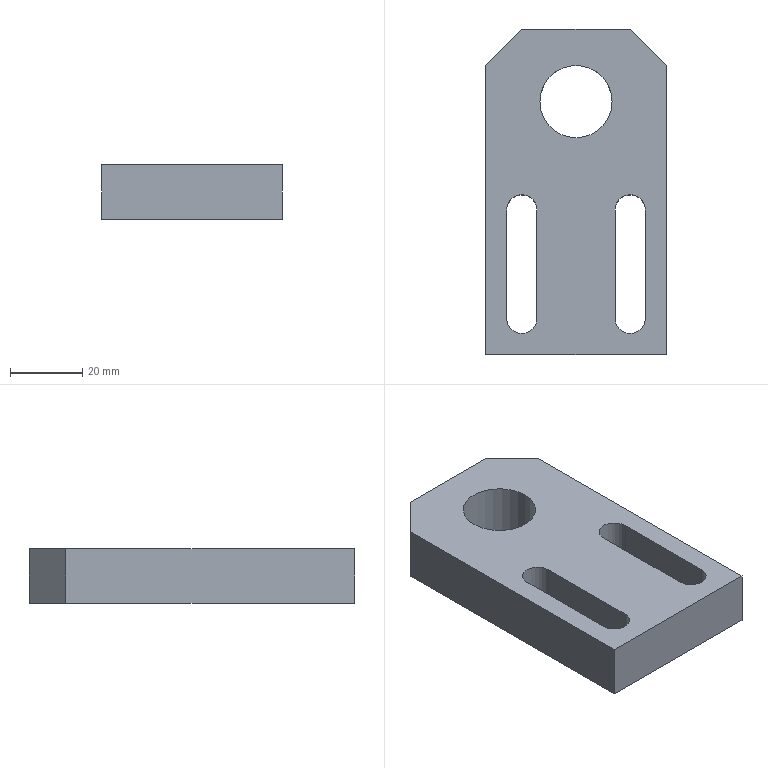Part | SolidWorks | features BaseBody 1 | 1 solid | 18 faces | box 50 x 90 x 15 mm | volume 52065 mm3 | plane 12 | cylinder 6 | commonest cylinder face diameters 8.4 x4 20 x2
STEP:
#1=CARTESIAN_POINT('',(-10.,20.,0.));
#2=VERTEX_POINT('',#1);
#3=CARTESIAN_POINT('',(10.,20.,0.));
#4=VERTEX_POINT('',#3);
#5=CARTESIAN_POINT('',(0.,20.,0.));
#6=DIRECTION('',(0.,0.,1.));
#7=DIRECTION('',(1.,0.,0.));
#8=AXIS2_PLACEMENT_3D('',#5,#6,#7);
#9=CIRCLE('',#8,10.);
#10=EDGE_CURVE('',#2,#4,#9,.T.);
#11=ORIENTED_EDGE('',*,*,#10,.F.);
#12=CARTESIAN_POINT('',(-10.,20.,15.));
#13=VERTEX_POINT('',#12);
#14=CARTESIAN_POINT('',(-10.,20.,0.));
#15=DIRECTION('',(0.,0.,1.));
#16=VECTOR('',#15,1000.);
#17=LINE('',#14,#16);
#18=EDGE_CURVE('',#2,#13,#17,.T.);
#19=ORIENTED_EDGE('',*,*,#18,.T.);
#20=CARTESIAN_POINT('',(10.,20.,15.));
#21=VERTEX_POINT('',#20);
#22=CARTESIAN_POINT('',(0.,20.,15.));
#23=DIRECTION('',(0.,0.,1.));
#24=DIRECTION('',(1.,0.,0.));
#25=AXIS2_PLACEMENT_3D('',#22,#23,#24);
#26=CIRCLE('',#25,10.);
#27=EDGE_CURVE('',#13,#21,#26,.T.);
#28=ORIENTED_EDGE('',*,*,#27,.T.);
#29=CARTESIAN_POINT('',(10.,20.,0.));
#30=DIRECTION('',(0.,0.,1.));
#31=VECTOR('',#30,1000.);
#32=LINE('',#29,#31);
#33=EDGE_CURVE('',#4,#21,#32,.T.);
#34=ORIENTED_EDGE('',*,*,#33,.F.);
#35=EDGE_LOOP('',(#11,#19,#28,#34));
#36=FACE_OUTER_BOUND('',#35,.T.);
#37=CARTESIAN_POINT('',(0.,20.,0.));
#38=DIRECTION('',(0.,0.,1.));
#39=DIRECTION('',(1.,0.,0.));
#40=AXIS2_PLACEMENT_3D('',#37,#38,#39);
#41=CYLINDRICAL_SURFACE('',#40,10.);
#42=ADVANCED_FACE('',(#36),#41,.F.);
#43=CARTESIAN_POINT('',(19.2,-40.,15.));
#44=VERTEX_POINT('',#43);
#45=CARTESIAN_POINT('',(19.2,-10.,15.));
#46=VERTEX_POINT('',#45);
#47=CARTESIAN_POINT('',(19.2,-40.,15.));
#48=DIRECTION('',(0.,1.,0.));
#49=VECTOR('',#48,1000.);
#50=LINE('',#47,#49);
#51=EDGE_CURVE('',#44,#46,#50,.T.);
#52=ORIENTED_EDGE('',*,*,#51,.T.);
#53=CARTESIAN_POINT('',(19.2,-10.,0.));
#54=VERTEX_POINT('',#53);
#55=CARTESIAN_POINT('',(19.2,-10.,0.));
#56=DIRECTION('',(0.,0.,1.));
#57=VECTOR('',#56,1000.);
#58=LINE('',#55,#57);
#59=EDGE_CURVE('',#54,#46,#58,.T.);
#60=ORIENTED_EDGE('',*,*,#59,.F.);
#61=CARTESIAN_POINT('',(19.2,-40.,0.));
#62=VERTEX_POINT('',#61);
#63=CARTESIAN_POINT('',(19.2,-40.,0.));
#64=DIRECTION('',(0.,1.,0.));
#65=VECTOR('',#64,1000.);
#66=LINE('',#63,#65);
#67=EDGE_CURVE('',#62,#54,#66,.T.);
#68=ORIENTED_EDGE('',*,*,#67,.F.);
#69=CARTESIAN_POINT('',(19.2,-40.,0.));
#70=DIRECTION('',(0.,0.,1.));
#71=VECTOR('',#70,1000.);
#72=LINE('',#69,#71);
#73=EDGE_CURVE('',#62,#44,#72,.T.);
#74=ORIENTED_EDGE('',*,*,#73,.T.);
#75=EDGE_LOOP('',(#52,#60,#68,#74));
#76=FACE_OUTER_BOUND('',#75,.T.);
#77=CARTESIAN_POINT('',(19.2,-40.,0.));
#78=DIRECTION('',(1.,0.,0.));
#79=DIRECTION('',(0.,1.,0.));
#80=AXIS2_PLACEMENT_3D('',#77,#78,#79);
#81=PLANE('',#80);
#82=ADVANCED_FACE('',(#76),#81,.F.);
#83=CARTESIAN_POINT('',(10.8,-10.,15.));
#84=VERTEX_POINT('',#83);
#85=CARTESIAN_POINT('',(15.,-10.,15.));
#86=DIRECTION('',(0.,0.,1.));
#87=DIRECTION('',(1.,0.,0.));
#88=AXIS2_PLACEMENT_3D('',#85,#86,#87);
#89=CIRCLE('',#88,4.2);
#90=EDGE_CURVE('',#46,#84,#89,.T.);
#91=ORIENTED_EDGE('',*,*,#90,.T.);
#92=CARTESIAN_POINT('',(10.8,-10.,0.));
#93=VERTEX_POINT('',#92);
#94=CARTESIAN_POINT('',(10.8,-10.,0.));
#95=DIRECTION('',(0.,0.,1.));
#96=VECTOR('',#95,1000.);
#97=LINE('',#94,#96);
#98=EDGE_CURVE('',#93,#84,#97,.T.);
#99=ORIENTED_EDGE('',*,*,#98,.F.);
#100=CARTESIAN_POINT('',(15.,-10.,0.));
#101=DIRECTION('',(0.,0.,1.));
#102=DIRECTION('',(1.,0.,0.));
#103=AXIS2_PLACEMENT_3D('',#100,#101,#102);
#104=CIRCLE('',#103,4.2);
#105=EDGE_CURVE('',#54,#93,#104,.T.);
#106=ORIENTED_EDGE('',*,*,#105,.F.);
#107=ORIENTED_EDGE('',*,*,#59,.T.);
#108=EDGE_LOOP('',(#91,#99,#106,#107));
#109=FACE_OUTER_BOUND('',#108,.T.);
#110=CARTESIAN_POINT('',(15.,-10.,0.));
#111=DIRECTION('',(0.,0.,1.));
#112=DIRECTION('',(1.,0.,0.));
#113=AXIS2_PLACEMENT_3D('',#110,#111,#112);
#114=CYLINDRICAL_SURFACE('',#113,4.2);
#115=ADVANCED_FACE('',(#109),#114,.F.);
#116=CARTESIAN_POINT('',(10.8,-40.,15.));
#117=VERTEX_POINT('',#116);
#118=CARTESIAN_POINT('',(10.8,-40.,15.));
#119=DIRECTION('',(0.,-1.,0.));
#120=VECTOR('',#119,1000.);
#121=LINE('',#118,#120);
#122=EDGE_CURVE('',#84,#117,#121,.T.);
#123=ORIENTED_EDGE('',*,*,#122,.T.);
#124=CARTESIAN_POINT('',(10.8,-40.,0.));
#125=VERTEX_POINT('',#124);
#126=CARTESIAN_POINT('',(10.8,-40.,0.));
#127=DIRECTION('',(0.,0.,1.));
#128=VECTOR('',#127,1000.);
#129=LINE('',#126,#128);
#130=EDGE_CURVE('',#125,#117,#129,.T.);
#131=ORIENTED_EDGE('',*,*,#130,.F.);
#132=CARTESIAN_POINT('',(10.8,-40.,0.));
#133=DIRECTION('',(0.,-1.,0.));
#134=VECTOR('',#133,1000.);
#135=LINE('',#132,#134);
#136=EDGE_CURVE('',#93,#125,#135,.T.);
#137=ORIENTED_EDGE('',*,*,#136,.F.);
#138=ORIENTED_EDGE('',*,*,#98,.T.);
#139=EDGE_LOOP('',(#123,#131,#137,#138));
#140=FACE_OUTER_BOUND('',#139,.T.);
#141=CARTESIAN_POINT('',(10.8,-40.,0.));
#142=DIRECTION('',(-1.,0.,0.));
#143=DIRECTION('',(0.,1.,0.));
#144=AXIS2_PLACEMENT_3D('',#141,#142,#143);
#145=PLANE('',#144);
#146=ADVANCED_FACE('',(#140),#145,.F.);
#147=CARTESIAN_POINT('',(15.,-40.,15.));
#148=DIRECTION('',(0.,0.,1.));
#149=DIRECTION('',(1.,0.,0.));
#150=AXIS2_PLACEMENT_3D('',#147,#148,#149);
#151=CIRCLE('',#150,4.2);
#152=EDGE_CURVE('',#117,#44,#151,.T.);
#153=ORIENTED_EDGE('',*,*,#152,.T.);
#154=ORIENTED_EDGE('',*,*,#73,.F.);
#155=CARTESIAN_POINT('',(15.,-40.,0.));
#156=DIRECTION('',(0.,0.,1.));
#157=DIRECTION('',(1.,0.,0.));
#158=AXIS2_PLACEMENT_3D('',#155,#156,#157);
#159=CIRCLE('',#158,4.2);
#160=EDGE_CURVE('',#125,#62,#159,.T.);
#161=ORIENTED_EDGE('',*,*,#160,.F.);
#162=ORIENTED_EDGE('',*,*,#130,.T.);
#163=EDGE_LOOP('',(#153,#154,#161,#162));
#164=FACE_OUTER_BOUND('',#163,.T.);
#165=CARTESIAN_POINT('',(15.,-40.,0.));
#166=DIRECTION('',(0.,0.,1.));
#167=DIRECTION('',(1.,0.,0.));
#168=AXIS2_PLACEMENT_3D('',#165,#166,#167);
#169=CYLINDRICAL_SURFACE('',#168,4.2);
#170=ADVANCED_FACE('',(#164),#169,.F.);
#171=CARTESIAN_POINT('',(-10.8,-40.,15.));
#172=VERTEX_POINT('',#171);
#173=CARTESIAN_POINT('',(-10.8,-10.,15.));
#174=VERTEX_POINT('',#173);
#175=CARTESIAN_POINT('',(-10.8,-40.,15.));
#176=DIRECTION('',(0.,1.,0.));
#177=VECTOR('',#176,1000.);
#178=LINE('',#175,#177);
#179=EDGE_CURVE('',#172,#174,#178,.T.);
#180=ORIENTED_EDGE('',*,*,#179,.T.);
#181=CARTESIAN_POINT('',(-10.8,-10.,0.));
#182=VERTEX_POINT('',#181);
#183=CARTESIAN_POINT('',(-10.8,-10.,0.));
#184=DIRECTION('',(0.,0.,1.));
#185=VECTOR('',#184,1000.);
#186=LINE('',#183,#185);
#187=EDGE_CURVE('',#182,#174,#186,.T.);
#188=ORIENTED_EDGE('',*,*,#187,.F.);
#189=CARTESIAN_POINT('',(-10.8,-40.,0.));
#190=VERTEX_POINT('',#189);
#191=CARTESIAN_POINT('',(-10.8,-40.,0.));
#192=DIRECTION('',(0.,1.,0.));
#193=VECTOR('',#192,1000.);
#194=LINE('',#191,#193);
#195=EDGE_CURVE('',#190,#182,#194,.T.);
#196=ORIENTED_EDGE('',*,*,#195,.F.);
#197=CARTESIAN_POINT('',(-10.8,-40.,0.));
#198=DIRECTION('',(0.,0.,1.));
#199=VECTOR('',#198,1000.);
#200=LINE('',#197,#199);
#201=EDGE_CURVE('',#190,#172,#200,.T.);
#202=ORIENTED_EDGE('',*,*,#201,.T.);
#203=EDGE_LOOP('',(#180,#188,#196,#202));
#204=FACE_OUTER_BOUND('',#203,.T.);
#205=CARTESIAN_POINT('',(-10.8,-40.,0.));
#206=DIRECTION('',(1.,0.,0.));
#207=DIRECTION('',(0.,1.,0.));
#208=AXIS2_PLACEMENT_3D('',#205,#206,#207);
#209=PLANE('',#208);
#210=ADVANCED_FACE('',(#204),#209,.F.);
#211=CARTESIAN_POINT('',(-19.2,-10.,15.));
#212=VERTEX_POINT('',#211);
#213=CARTESIAN_POINT('',(-15.,-10.,15.));
#214=DIRECTION('',(0.,0.,1.));
#215=DIRECTION('',(1.,0.,0.));
#216=AXIS2_PLACEMENT_3D('',#213,#214,#215);
#217=CIRCLE('',#216,4.2);
#218=EDGE_CURVE('',#174,#212,#217,.T.);
#219=ORIENTED_EDGE('',*,*,#218,.T.);
#220=CARTESIAN_POINT('',(-19.2,-10.,0.));
#221=VERTEX_POINT('',#220);
#222=CARTESIAN_POINT('',(-19.2,-10.,0.));
#223=DIRECTION('',(0.,0.,1.));
#224=VECTOR('',#223,1000.);
#225=LINE('',#222,#224);
#226=EDGE_CURVE('',#221,#212,#225,.T.);
#227=ORIENTED_EDGE('',*,*,#226,.F.);
#228=CARTESIAN_POINT('',(-15.,-10.,0.));
#229=DIRECTION('',(0.,0.,1.));
#230=DIRECTION('',(1.,0.,0.));
#231=AXIS2_PLACEMENT_3D('',#228,#229,#230);
#232=CIRCLE('',#231,4.2);
#233=EDGE_CURVE('',#182,#221,#232,.T.);
#234=ORIENTED_EDGE('',*,*,#233,.F.);
#235=ORIENTED_EDGE('',*,*,#187,.T.);
#236=EDGE_LOOP('',(#219,#227,#234,#235));
#237=FACE_OUTER_BOUND('',#236,.T.);
#238=CARTESIAN_POINT('',(-15.,-10.,0.));
#239=DIRECTION('',(0.,0.,1.));
#240=DIRECTION('',(1.,0.,0.));
#241=AXIS2_PLACEMENT_3D('',#238,#239,#240);
#242=CYLINDRICAL_SURFACE('',#241,4.2);
#243=ADVANCED_FACE('',(#237),#242,.F.);
#244=CARTESIAN_POINT('',(-19.2,-40.,15.));
#245=VERTEX_POINT('',#244);
#246=CARTESIAN_POINT('',(-19.2,-40.,15.));
#247=DIRECTION('',(0.,-1.,0.));
#248=VECTOR('',#247,1000.);
#249=LINE('',#246,#248);
#250=EDGE_CURVE('',#212,#245,#249,.T.);
#251=ORIENTED_EDGE('',*,*,#250,.T.);
#252=CARTESIAN_POINT('',(-19.2,-40.,0.));
#253=VERTEX_POINT('',#252);
#254=CARTESIAN_POINT('',(-19.2,-40.,0.));
#255=DIRECTION('',(0.,0.,1.));
#256=VECTOR('',#255,1000.);
#257=LINE('',#254,#256);
#258=EDGE_CURVE('',#253,#245,#257,.T.);
#259=ORIENTED_EDGE('',*,*,#258,.F.);
#260=CARTESIAN_POINT('',(-19.2,-40.,0.));
#261=DIRECTION('',(0.,-1.,0.));
#262=VECTOR('',#261,1000.);
#263=LINE('',#260,#262);
#264=EDGE_CURVE('',#221,#253,#263,.T.);
#265=ORIENTED_EDGE('',*,*,#264,.F.);
#266=ORIENTED_EDGE('',*,*,#226,.T.);
#267=EDGE_LOOP('',(#251,#259,#265,#266));
#268=FACE_OUTER_BOUND('',#267,.T.);
#269=CARTESIAN_POINT('',(-19.2,-40.,0.));
#270=DIRECTION('',(-1.,0.,0.));
#271=DIRECTION('',(0.,1.,0.));
#272=AXIS2_PLACEMENT_3D('',#269,#270,#271);
#273=PLANE('',#272);
#274=ADVANCED_FACE('',(#268),#273,.F.);
#275=CARTESIAN_POINT('',(-15.,-40.,15.));
#276=DIRECTION('',(0.,0.,1.));
#277=DIRECTION('',(1.,0.,0.));
#278=AXIS2_PLACEMENT_3D('',#275,#276,#277);
#279=CIRCLE('',#278,4.2);
#280=EDGE_CURVE('',#245,#172,#279,.T.);
#281=ORIENTED_EDGE('',*,*,#280,.T.);
#282=ORIENTED_EDGE('',*,*,#201,.F.);
#283=CARTESIAN_POINT('',(-15.,-40.,0.));
#284=DIRECTION('',(0.,0.,1.));
#285=DIRECTION('',(1.,0.,0.));
#286=AXIS2_PLACEMENT_3D('',#283,#284,#285);
#287=CIRCLE('',#286,4.2);
#288=EDGE_CURVE('',#253,#190,#287,.T.);
#289=ORIENTED_EDGE('',*,*,#288,.F.);
#290=ORIENTED_EDGE('',*,*,#258,.T.);
#291=EDGE_LOOP('',(#281,#282,#289,#290));
#292=FACE_OUTER_BOUND('',#291,.T.);
#293=CARTESIAN_POINT('',(-15.,-40.,0.));
#294=DIRECTION('',(0.,0.,1.));
#295=DIRECTION('',(1.,0.,0.));
#296=AXIS2_PLACEMENT_3D('',#293,#294,#295);
#297=CYLINDRICAL_SURFACE('',#296,4.2);
#298=ADVANCED_FACE('',(#292),#297,.F.);
#299=CARTESIAN_POINT('',(-25.,-50.,15.));
#300=VERTEX_POINT('',#299);
#301=CARTESIAN_POINT('',(-25.,-50.,0.));
#302=VERTEX_POINT('',#301);
#303=CARTESIAN_POINT('',(-25.,-50.,15.));
#304=DIRECTION('',(0.,0.,-1.));
#305=VECTOR('',#304,1000.);
#306=LINE('',#303,#305);
#307=EDGE_CURVE('',#300,#302,#306,.T.);
#308=ORIENTED_EDGE('',*,*,#307,.T.);
#309=CARTESIAN_POINT('',(25.,-50.,0.));
#310=VERTEX_POINT('',#309);
#311=CARTESIAN_POINT('',(-25.,-50.,0.));
#312=DIRECTION('',(1.,0.,0.));
#313=VECTOR('',#312,1000.);
#314=LINE('',#311,#313);
#315=EDGE_CURVE('',#302,#310,#314,.T.);
#316=ORIENTED_EDGE('',*,*,#315,.T.);
#317=CARTESIAN_POINT('',(25.,-50.,15.));
#318=VERTEX_POINT('',#317);
#319=CARTESIAN_POINT('',(25.,-50.,0.));
#320=DIRECTION('',(0.,0.,1.));
#321=VECTOR('',#320,1000.);
#322=LINE('',#319,#321);
#323=EDGE_CURVE('',#310,#318,#322,.T.);
#324=ORIENTED_EDGE('',*,*,#323,.T.);
#325=CARTESIAN_POINT('',(25.,-50.,15.));
#326=DIRECTION('',(-1.,0.,0.));
#327=VECTOR('',#326,1000.);
#328=LINE('',#325,#327);
#329=EDGE_CURVE('',#318,#300,#328,.T.);
#330=ORIENTED_EDGE('',*,*,#329,.T.);
#331=EDGE_LOOP('',(#308,#316,#324,#330));
#332=FACE_OUTER_BOUND('',#331,.T.);
#333=CARTESIAN_POINT('',(0.,-50.,0.));
#334=DIRECTION('',(0.,-1.,0.));
#335=DIRECTION('',(0.,0.,-1.));
#336=AXIS2_PLACEMENT_3D('',#333,#334,#335);
#337=PLANE('',#336);
#338=ADVANCED_FACE('',(#332),#337,.T.);
#339=CARTESIAN_POINT('',(-15.,40.,15.));
#340=VERTEX_POINT('',#339);
#341=CARTESIAN_POINT('',(-25.,30.,15.));
#342=VERTEX_POINT('',#341);
#343=CARTESIAN_POINT('',(-27.5,27.5,15.));
#344=DIRECTION('',(-0.7071,-0.7071,0.));
#345=VECTOR('',#344,1000.);
#346=LINE('',#343,#345);
#347=EDGE_CURVE('',#340,#342,#346,.T.);
#348=ORIENTED_EDGE('',*,*,#347,.F.);
#349=CARTESIAN_POINT('',(-15.,40.,0.));
#350=VERTEX_POINT('',#349);
#351=CARTESIAN_POINT('',(-15.,40.,15.));
#352=DIRECTION('',(0.,0.,1.));
#353=VECTOR('',#352,1000.);
#354=LINE('',#351,#353);
#355=EDGE_CURVE('',#350,#340,#354,.T.);
#356=ORIENTED_EDGE('',*,*,#355,.F.);
#357=CARTESIAN_POINT('',(-25.,30.,0.));
#358=VERTEX_POINT('',#357);
#359=CARTESIAN_POINT('',(-25.,30.,0.));
#360=DIRECTION('',(0.7071,0.7071,0.));
#361=VECTOR('',#360,1000.);
#362=LINE('',#359,#361);
#363=EDGE_CURVE('',#358,#350,#362,.T.);
#364=ORIENTED_EDGE('',*,*,#363,.F.);
#365=CARTESIAN_POINT('',(-25.,30.,15.));
#366=DIRECTION('',(0.,0.,-1.));
#367=VECTOR('',#366,1000.);
#368=LINE('',#365,#367);
#369=EDGE_CURVE('',#342,#358,#368,.T.);
#370=ORIENTED_EDGE('',*,*,#369,.F.);
#371=EDGE_LOOP('',(#348,#356,#364,#370));
#372=FACE_OUTER_BOUND('',#371,.T.);
#373=CARTESIAN_POINT('',(-25.,30.,15.));
#374=DIRECTION('',(0.7071,-0.7071,0.));
#375=DIRECTION('',(0.,0.,-1.));
#376=AXIS2_PLACEMENT_3D('',#373,#374,#375);
#377=PLANE('',#376);
#378=ADVANCED_FACE('',(#372),#377,.F.);
#379=CARTESIAN_POINT('',(25.,30.,15.));
#380=VERTEX_POINT('',#379);
#381=CARTESIAN_POINT('',(15.,40.,15.));
#382=VERTEX_POINT('',#381);
#383=CARTESIAN_POINT('',(27.5,27.5,15.));
#384=DIRECTION('',(-0.7071,0.7071,0.));
#385=VECTOR('',#384,1000.);
#386=LINE('',#383,#385);
#387=EDGE_CURVE('',#380,#382,#386,.T.);
#388=ORIENTED_EDGE('',*,*,#387,.F.);
#389=CARTESIAN_POINT('',(25.,30.,0.));
#390=VERTEX_POINT('',#389);
#391=CARTESIAN_POINT('',(25.,30.,15.));
#392=DIRECTION('',(0.,0.,1.));
#393=VECTOR('',#392,1000.);
#394=LINE('',#391,#393);
#395=EDGE_CURVE('',#390,#380,#394,.T.);
#396=ORIENTED_EDGE('',*,*,#395,.F.);
#397=CARTESIAN_POINT('',(15.,40.,0.));
#398=VERTEX_POINT('',#397);
#399=CARTESIAN_POINT('',(15.,40.,0.));
#400=DIRECTION('',(0.7071,-0.7071,0.));
#401=VECTOR('',#400,1000.);
#402=LINE('',#399,#401);
#403=EDGE_CURVE('',#398,#390,#402,.T.);
#404=ORIENTED_EDGE('',*,*,#403,.F.);
#405=CARTESIAN_POINT('',(15.,40.,15.));
#406=DIRECTION('',(0.,0.,-1.));
#407=VECTOR('',#406,1000.);
#408=LINE('',#405,#407);
#409=EDGE_CURVE('',#382,#398,#408,.T.);
#410=ORIENTED_EDGE('',*,*,#409,.F.);
#411=EDGE_LOOP('',(#388,#396,#404,#410));
#412=FACE_OUTER_BOUND('',#411,.T.);
#413=CARTESIAN_POINT('',(15.,40.,15.));
#414=DIRECTION('',(-0.7071,-0.7071,0.));
#415=DIRECTION('',(-0.7071,0.7071,0.));
#416=AXIS2_PLACEMENT_3D('',#413,#414,#415);
#417=PLANE('',#416);
#418=ADVANCED_FACE('',(#412),#417,.F.);
#419=CARTESIAN_POINT('',(0.,20.,0.));
#420=DIRECTION('',(0.,0.,1.));
#421=DIRECTION('',(1.,0.,0.));
#422=AXIS2_PLACEMENT_3D('',#419,#420,#421);
#423=CIRCLE('',#422,10.);
#424=EDGE_CURVE('',#4,#2,#423,.T.);
#425=ORIENTED_EDGE('',*,*,#424,.T.);
#426=ORIENTED_EDGE('',*,*,#10,.T.);
#427=EDGE_LOOP('',(#425,#426));
#428=FACE_BOUND('',#427,.T.);
#429=ORIENTED_EDGE('',*,*,#264,.T.);
#430=ORIENTED_EDGE('',*,*,#288,.T.);
#431=ORIENTED_EDGE('',*,*,#195,.T.);
#432=ORIENTED_EDGE('',*,*,#233,.T.);
#433=EDGE_LOOP('',(#429,#430,#431,#432));
#434=FACE_BOUND('',#433,.T.);
#435=ORIENTED_EDGE('',*,*,#136,.T.);
#436=ORIENTED_EDGE('',*,*,#160,.T.);
#437=ORIENTED_EDGE('',*,*,#67,.T.);
#438=ORIENTED_EDGE('',*,*,#105,.T.);
#439=EDGE_LOOP('',(#435,#436,#437,#438));
#440=FACE_BOUND('',#439,.T.);
#441=CARTESIAN_POINT('',(-25.,40.,0.));
#442=DIRECTION('',(-1.,0.,0.));
#443=VECTOR('',#442,1000.);
#444=LINE('',#441,#443);
#445=EDGE_CURVE('',#398,#350,#444,.T.);
#446=ORIENTED_EDGE('',*,*,#445,.F.);
#447=ORIENTED_EDGE('',*,*,#403,.T.);
#448=CARTESIAN_POINT('',(25.,40.,0.));
#449=DIRECTION('',(0.,1.,0.));
#450=VECTOR('',#449,1000.);
#451=LINE('',#448,#450);
#452=EDGE_CURVE('',#310,#390,#451,.T.);
#453=ORIENTED_EDGE('',*,*,#452,.F.);
#454=ORIENTED_EDGE('',*,*,#315,.F.);
#455=CARTESIAN_POINT('',(-25.,40.,0.));
#456=DIRECTION('',(0.,-1.,0.));
#457=VECTOR('',#456,1000.);
#458=LINE('',#455,#457);
#459=EDGE_CURVE('',#358,#302,#458,.T.);
#460=ORIENTED_EDGE('',*,*,#459,.F.);
#461=ORIENTED_EDGE('',*,*,#363,.T.);
#462=EDGE_LOOP('',(#446,#447,#453,#454,#460,#461));
#463=FACE_OUTER_BOUND('',#462,.T.);
#464=CARTESIAN_POINT('',(0.,0.,0.));
#465=DIRECTION('',(0.,0.,1.));
#466=DIRECTION('',(1.,0.,0.));
#467=AXIS2_PLACEMENT_3D('',#464,#465,#466);
#468=PLANE('',#467);
#469=ADVANCED_FACE('',(#428,#434,#440,#463),#468,.F.);
#470=CARTESIAN_POINT('',(0.,20.,15.));
#471=DIRECTION('',(0.,0.,1.));
#472=DIRECTION('',(1.,0.,0.));
#473=AXIS2_PLACEMENT_3D('',#470,#471,#472);
#474=CIRCLE('',#473,10.);
#475=EDGE_CURVE('',#21,#13,#474,.T.);
#476=ORIENTED_EDGE('',*,*,#475,.F.);
#477=ORIENTED_EDGE('',*,*,#27,.F.);
#478=EDGE_LOOP('',(#476,#477));
#479=FACE_BOUND('',#478,.T.);
#480=ORIENTED_EDGE('',*,*,#280,.F.);
#481=ORIENTED_EDGE('',*,*,#250,.F.);
#482=ORIENTED_EDGE('',*,*,#218,.F.);
#483=ORIENTED_EDGE('',*,*,#179,.F.);
#484=EDGE_LOOP('',(#480,#481,#482,#483));
#485=FACE_BOUND('',#484,.T.);
#486=ORIENTED_EDGE('',*,*,#152,.F.);
#487=ORIENTED_EDGE('',*,*,#122,.F.);
#488=ORIENTED_EDGE('',*,*,#90,.F.);
#489=ORIENTED_EDGE('',*,*,#51,.F.);
#490=EDGE_LOOP('',(#486,#487,#488,#489));
#491=FACE_BOUND('',#490,.T.);
#492=CARTESIAN_POINT('',(25.,40.,15.));
#493=DIRECTION('',(0.,1.,0.));
#494=VECTOR('',#493,1000.);
#495=LINE('',#492,#494);
#496=EDGE_CURVE('',#318,#380,#495,.T.);
#497=ORIENTED_EDGE('',*,*,#496,.T.);
#498=ORIENTED_EDGE('',*,*,#387,.T.);
#499=CARTESIAN_POINT('',(-25.,40.,15.));
#500=DIRECTION('',(-1.,0.,0.));
#501=VECTOR('',#500,1000.);
#502=LINE('',#499,#501);
#503=EDGE_CURVE('',#382,#340,#502,.T.);
#504=ORIENTED_EDGE('',*,*,#503,.T.);
#505=ORIENTED_EDGE('',*,*,#347,.T.);
#506=CARTESIAN_POINT('',(-25.,40.,15.));
#507=DIRECTION('',(0.,-1.,0.));
#508=VECTOR('',#507,1000.);
#509=LINE('',#506,#508);
#510=EDGE_CURVE('',#342,#300,#509,.T.);
#511=ORIENTED_EDGE('',*,*,#510,.T.);
#512=ORIENTED_EDGE('',*,*,#329,.F.);
#513=EDGE_LOOP('',(#497,#498,#504,#505,#511,#512));
#514=FACE_OUTER_BOUND('',#513,.T.);
#515=CARTESIAN_POINT('',(0.,0.,15.));
#516=DIRECTION('',(0.,0.,1.));
#517=DIRECTION('',(1.,0.,0.));
#518=AXIS2_PLACEMENT_3D('',#515,#516,#517);
#519=PLANE('',#518);
#520=ADVANCED_FACE('',(#479,#485,#491,#514),#519,.T.);
#521=ORIENTED_EDGE('',*,*,#510,.F.);
#522=ORIENTED_EDGE('',*,*,#369,.T.);
#523=ORIENTED_EDGE('',*,*,#459,.T.);
#524=ORIENTED_EDGE('',*,*,#307,.F.);
#525=EDGE_LOOP('',(#521,#522,#523,#524));
#526=FACE_OUTER_BOUND('',#525,.T.);
#527=CARTESIAN_POINT('',(-25.,40.,15.));
#528=DIRECTION('',(1.,0.,0.));
#529=DIRECTION('',(0.,1.,0.));
#530=AXIS2_PLACEMENT_3D('',#527,#528,#529);
#531=PLANE('',#530);
#532=ADVANCED_FACE('',(#526),#531,.F.);
#533=ORIENTED_EDGE('',*,*,#503,.F.);
#534=ORIENTED_EDGE('',*,*,#409,.T.);
#535=ORIENTED_EDGE('',*,*,#445,.T.);
#536=ORIENTED_EDGE('',*,*,#355,.T.);
#537=EDGE_LOOP('',(#533,#534,#535,#536));
#538=FACE_OUTER_BOUND('',#537,.T.);
#539=CARTESIAN_POINT('',(-25.,40.,15.));
#540=DIRECTION('',(0.,-1.,0.));
#541=DIRECTION('',(0.,0.,-1.));
#542=AXIS2_PLACEMENT_3D('',#539,#540,#541);
#543=PLANE('',#542);
#544=ADVANCED_FACE('',(#538),#543,.F.);
#545=ORIENTED_EDGE('',*,*,#452,.T.);
#546=ORIENTED_EDGE('',*,*,#395,.T.);
#547=ORIENTED_EDGE('',*,*,#496,.F.);
#548=ORIENTED_EDGE('',*,*,#323,.F.);
#549=EDGE_LOOP('',(#545,#546,#547,#548));
#550=FACE_OUTER_BOUND('',#549,.T.);
#551=CARTESIAN_POINT('',(25.,40.,15.));
#552=DIRECTION('',(-1.,0.,0.));
#553=DIRECTION('',(0.,1.,0.));
#554=AXIS2_PLACEMENT_3D('',#551,#552,#553);
#555=PLANE('',#554);
#556=ADVANCED_FACE('',(#550),#555,.F.);
#557=ORIENTED_EDGE('',*,*,#18,.F.);
#558=ORIENTED_EDGE('',*,*,#424,.F.);
#559=ORIENTED_EDGE('',*,*,#33,.T.);
#560=ORIENTED_EDGE('',*,*,#475,.T.);
#561=EDGE_LOOP('',(#557,#558,#559,#560));
#562=FACE_OUTER_BOUND('',#561,.T.);
#563=CARTESIAN_POINT('',(0.,20.,0.));
#564=DIRECTION('',(0.,0.,1.));
#565=DIRECTION('',(1.,0.,0.));
#566=AXIS2_PLACEMENT_3D('',#563,#564,#565);
#567=CYLINDRICAL_SURFACE('',#566,10.);
#568=ADVANCED_FACE('',(#562),#567,.F.);
#569=CLOSED_SHELL('',(#42,#82,#115,#146,#170,#210,#243,#274,#298,#338,#378,#418,#469,#520,#532,#544,#556,#568));
#570=MANIFOLD_SOLID_BREP('',#569);
#571=CARTESIAN_POINT('',(0.,0.,0.));
#572=DIRECTION('',(0.,0.,1.));
#573=DIRECTION('',(1.,0.,0.));
#574=AXIS2_PLACEMENT_3D('',#571,#572,#573);
#575=(LENGTH_UNIT()NAMED_UNIT(*)SI_UNIT(.MILLI.,.METRE.));
#576=UNCERTAINTY_MEASURE_WITH_UNIT(LENGTH_MEASURE(0.00001),#575,'','');
#577=(NAMED_UNIT(*)PLANE_ANGLE_UNIT()SI_UNIT($,.RADIAN.));
#578=(NAMED_UNIT(*)SI_UNIT($,.STERADIAN.)SOLID_ANGLE_UNIT());
#579=(GEOMETRIC_REPRESENTATION_CONTEXT(3)GLOBAL_UNCERTAINTY_ASSIGNED_CONTEXT((#576))GLOBAL_UNIT_ASSIGNED_CONTEXT((#575,#577,#578))REPRESENTATION_CONTEXT('',''));
#580=ADVANCED_BREP_SHAPE_REPRESENTATION('',(#570,#574),#579);